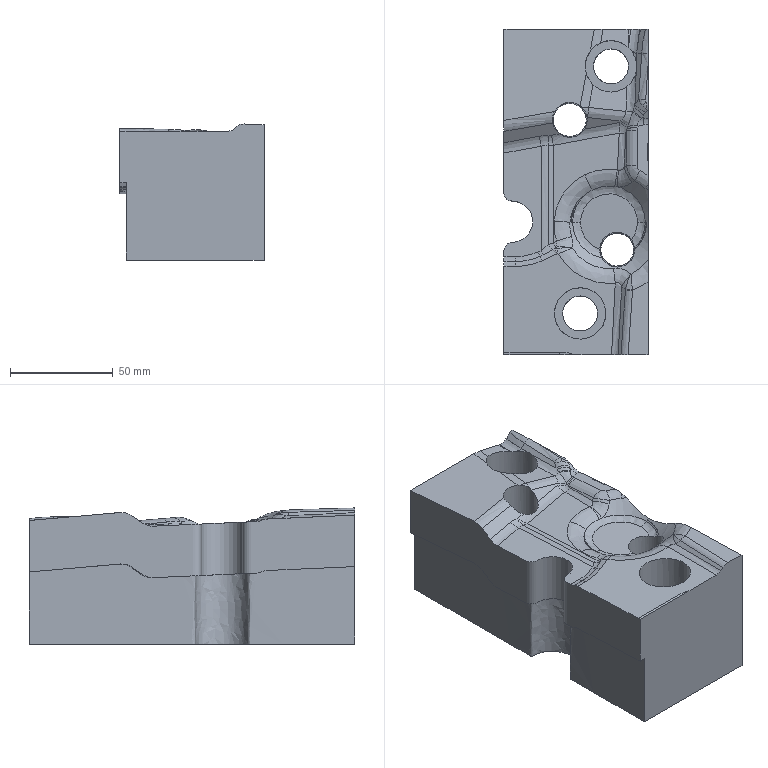Part | NX | features solid 2 | 1 solid | 125 faces | volume 576822 mm3 | spline 109 | plane 8 | cylinder 8 | commonest cylinder face diameters 17 x4 16 x2 25 x2